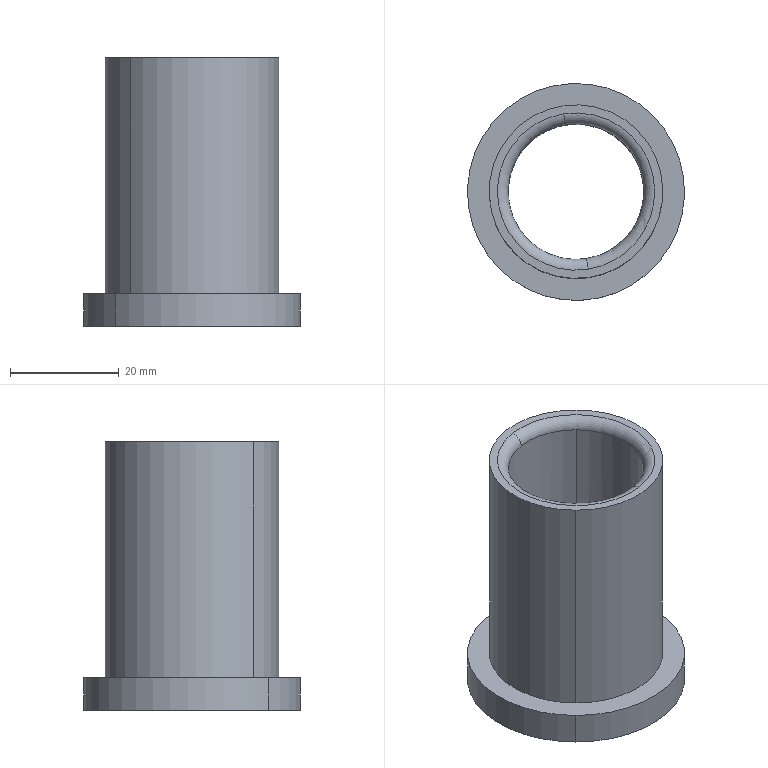Part | 1 solid | 11 faces | box 40 x 40 x 49.5 mm | volume 18157 mm3 | cylinder 6 | plane 3 | torus 2 | commonest cylinder face diameters 25 x2 32 x2 40 x2
STEP:
#1=CARTESIAN_POINT('',(0.,0.,0.));
#2=DIRECTION('',(0.,0.,1.));
#3=DIRECTION('',(1.,0.,0.));
#4=AXIS2_PLACEMENT_3D('',#1,#2,#3);
#5=CARTESIAN_POINT('',(-343.839,33.661,-238.55));
#6=VERTEX_POINT('',#5);
#7=CARTESIAN_POINT('',(-326.161,51.339,-238.55));
#8=VERTEX_POINT('',#7);
#9=CARTESIAN_POINT('',(-335.,42.5,-238.55));
#10=DIRECTION('',(0.,0.,1.));
#11=DIRECTION('',(0.7071,0.7071,0.));
#12=AXIS2_PLACEMENT_3D('',#9,#10,#11);
#13=CIRCLE('',#12,12.5);
#14=CARTESIAN_POINT('',(-335.,42.5,-200.318));
#15=DIRECTION('',(0.,0.,1.));
#16=DIRECTION('',(-0.7071,0.7071,0.));
#17=AXIS2_PLACEMENT_3D('',#14,#15,#16);
#18=CYLINDRICAL_SURFACE('',#17,12.5);
#19=CARTESIAN_POINT('',(-1.571,-38.232));
#20=DIRECTION('',(1.,0.));
#21=VECTOR('',#20,1.);
#22=LINE('',#19,#21);
#23=(GEOMETRIC_REPRESENTATION_CONTEXT(2)PARAMETRIC_REPRESENTATION_CONTEXT()REPRESENTATION_CONTEXT('',''));
#24=DEFINITIONAL_REPRESENTATION('',(#22),#23);
#25=PCURVE('',#18,#24);
#26=CARTESIAN_POINT('',(-320.858,28.358,-238.55));
#27=DIRECTION('',(0.,0.,-1.));
#28=DIRECTION('',(-0.7071,-0.7071,0.));
#29=AXIS2_PLACEMENT_3D('',#26,#27,#28);
#30=PLANE('',#29);
#31=CARTESIAN_POINT('',(-12.5,20.));
#32=CARTESIAN_POINT('',(-12.5,41.651));
#33=CARTESIAN_POINT('',(6.25,30.825));
#34=CARTESIAN_POINT('',(25.,20.));
#35=CARTESIAN_POINT('',(6.25,9.175));
#36=CARTESIAN_POINT('',(-12.5,-1.651));
#37=CARTESIAN_POINT('',(-12.5,20.));
#38=(BOUNDED_CURVE()B_SPLINE_CURVE(2,(#31,#32,#33,#34,#35,#36,#37),.UNSPECIFIED.,.T.,.F.)B_SPLINE_CURVE_WITH_KNOTS((1,2,2,2,2,1),(-2.094,0.,2.094,4.189,6.283,8.378),.UNSPECIFIED.)CURVE()GEOMETRIC_REPRESENTATION_ITEM()RATIONAL_B_SPLINE_CURVE((1.,0.5,1.,0.5,1.,0.5,1.))REPRESENTATION_ITEM(''));
#39=(GEOMETRIC_REPRESENTATION_CONTEXT(2)PARAMETRIC_REPRESENTATION_CONTEXT()REPRESENTATION_CONTEXT('',''));
#40=DEFINITIONAL_REPRESENTATION('',(#38),#39);
#41=PCURVE('',#30,#40);
#42=SURFACE_CURVE('',#13,(#25,#41),.PCURVE_S1.);
#43=EDGE_CURVE('',#6,#8,#42,.T.);
#44=ORIENTED_EDGE('',*,*,#43,.T.);
#45=CARTESIAN_POINT('',(-326.161,51.339,-191.05));
#46=VERTEX_POINT('',#45);
#47=CARTESIAN_POINT('',(-326.161,51.339,-238.55));
#48=DIRECTION('',(0.,0.,1.));
#49=VECTOR('',#48,1.);
#50=LINE('',#47,#49);
#51=CARTESIAN_POINT('',(4.712,-38.232));
#52=DIRECTION('',(0.,1.));
#53=VECTOR('',#52,1.);
#54=LINE('',#51,#53);
#55=(GEOMETRIC_REPRESENTATION_CONTEXT(2)PARAMETRIC_REPRESENTATION_CONTEXT()REPRESENTATION_CONTEXT('',''));
#56=DEFINITIONAL_REPRESENTATION('',(#54),#55);
#57=PCURVE('',#18,#56);
#58=CARTESIAN_POINT('',(-335.,42.5,-200.318));
#59=DIRECTION('',(0.,0.,1.));
#60=DIRECTION('',(0.7071,-0.7071,0.));
#61=AXIS2_PLACEMENT_3D('',#58,#59,#60);
#62=CYLINDRICAL_SURFACE('',#61,12.5);
#63=CARTESIAN_POINT('',(1.571,-38.232));
#64=DIRECTION('',(0.,1.));
#65=VECTOR('',#64,1.);
#66=LINE('',#63,#65);
#67=(GEOMETRIC_REPRESENTATION_CONTEXT(2)PARAMETRIC_REPRESENTATION_CONTEXT()REPRESENTATION_CONTEXT('',''));
#68=DEFINITIONAL_REPRESENTATION('',(#66),#67);
#69=PCURVE('',#62,#68);
#70=SURFACE_CURVE('',#50,(#57,#69),.PCURVE_S1.);
#71=EDGE_CURVE('',#8,#46,#70,.T.);
#72=ORIENTED_EDGE('',*,*,#71,.T.);
#73=CARTESIAN_POINT('',(-322.654,40.545,-191.05));
#74=VERTEX_POINT('',#73);
#75=CARTESIAN_POINT('',(-335.,42.5,-191.05));
#76=DIRECTION('',(0.,0.,-1.));
#77=DIRECTION('',(0.9877,-0.1564,0.));
#78=AXIS2_PLACEMENT_3D('',#75,#76,#77);
#79=CIRCLE('',#78,12.5);
#80=CARTESIAN_POINT('',(10.053,9.268));
#81=DIRECTION('',(-1.,0.));
#82=VECTOR('',#81,1.);
#83=LINE('',#80,#82);
#84=(GEOMETRIC_REPRESENTATION_CONTEXT(2)PARAMETRIC_REPRESENTATION_CONTEXT()REPRESENTATION_CONTEXT('',''));
#85=DEFINITIONAL_REPRESENTATION('',(#83),#84);
#86=PCURVE('',#18,#85);
#87=CARTESIAN_POINT('',(-335.,42.5,-191.05));
#88=DIRECTION('',(0.,0.,1.));
#89=DIRECTION('',(-0.9877,-0.1564,0.));
#90=AXIS2_PLACEMENT_3D('',#87,#88,#89);
#91=TOROIDAL_SURFACE('',#90,14.5,2.);
#92=CARTESIAN_POINT('',(9.111,3.142));
#93=DIRECTION('',(-1.,0.));
#94=VECTOR('',#93,1.);
#95=LINE('',#92,#94);
#96=(GEOMETRIC_REPRESENTATION_CONTEXT(2)PARAMETRIC_REPRESENTATION_CONTEXT()REPRESENTATION_CONTEXT('',''));
#97=DEFINITIONAL_REPRESENTATION('',(#95),#96);
#98=PCURVE('',#91,#97);
#99=SURFACE_CURVE('',#79,(#86,#98),.PCURVE_S1.);
#100=EDGE_CURVE('',#46,#74,#99,.T.);
#101=ORIENTED_EDGE('',*,*,#100,.T.);
#102=CARTESIAN_POINT('',(-333.044,30.154,-191.05));
#103=VERTEX_POINT('',#102);
#104=CARTESIAN_POINT('',(-335.,42.5,-191.05));
#105=DIRECTION('',(0.,0.,-1.));
#106=DIRECTION('',(0.9877,-0.1564,0.));
#107=AXIS2_PLACEMENT_3D('',#104,#105,#106);
#108=CIRCLE('',#107,12.5);
#109=CARTESIAN_POINT('',(3.77,9.268));
#110=DIRECTION('',(-1.,0.));
#111=VECTOR('',#110,1.);
#112=LINE('',#109,#111);
#113=(GEOMETRIC_REPRESENTATION_CONTEXT(2)PARAMETRIC_REPRESENTATION_CONTEXT()REPRESENTATION_CONTEXT('',''));
#114=DEFINITIONAL_REPRESENTATION('',(#112),#113);
#115=PCURVE('',#18,#114);
#116=CARTESIAN_POINT('',(2.827,3.142));
#117=DIRECTION('',(-1.,0.));
#118=VECTOR('',#117,1.);
#119=LINE('',#116,#118);
#120=(GEOMETRIC_REPRESENTATION_CONTEXT(2)PARAMETRIC_REPRESENTATION_CONTEXT()REPRESENTATION_CONTEXT('',''));
#121=DEFINITIONAL_REPRESENTATION('',(#119),#120);
#122=PCURVE('',#91,#121);
#123=SURFACE_CURVE('',#108,(#115,#122),.PCURVE_S1.);
#124=EDGE_CURVE('',#74,#103,#123,.T.);
#125=ORIENTED_EDGE('',*,*,#124,.T.);
#126=CARTESIAN_POINT('',(-343.839,33.661,-191.05));
#127=VERTEX_POINT('',#126);
#128=CARTESIAN_POINT('',(-335.,42.5,-191.05));
#129=DIRECTION('',(0.,0.,-1.));
#130=DIRECTION('',(0.9877,-0.1564,0.));
#131=AXIS2_PLACEMENT_3D('',#128,#129,#130);
#132=CIRCLE('',#131,12.5);
#133=CARTESIAN_POINT('',(3.77,9.268));
#134=DIRECTION('',(-1.,0.));
#135=VECTOR('',#134,1.);
#136=LINE('',#133,#135);
#137=(GEOMETRIC_REPRESENTATION_CONTEXT(2)PARAMETRIC_REPRESENTATION_CONTEXT()REPRESENTATION_CONTEXT('',''));
#138=DEFINITIONAL_REPRESENTATION('',(#136),#137);
#139=PCURVE('',#18,#138);
#140=CARTESIAN_POINT('',(-335.,42.5,-191.05));
#141=DIRECTION('',(0.,0.,1.));
#142=DIRECTION('',(0.9877,0.1564,0.));
#143=AXIS2_PLACEMENT_3D('',#140,#141,#142);
#144=TOROIDAL_SURFACE('',#143,14.5,2.);
#145=CARTESIAN_POINT('',(5.969,3.142));
#146=DIRECTION('',(-1.,0.));
#147=VECTOR('',#146,1.);
#148=LINE('',#145,#147);
#149=(GEOMETRIC_REPRESENTATION_CONTEXT(2)PARAMETRIC_REPRESENTATION_CONTEXT()REPRESENTATION_CONTEXT('',''));
#150=DEFINITIONAL_REPRESENTATION('',(#148),#149);
#151=PCURVE('',#144,#150);
#152=SURFACE_CURVE('',#132,(#139,#151),.PCURVE_S1.);
#153=EDGE_CURVE('',#103,#127,#152,.T.);
#154=ORIENTED_EDGE('',*,*,#153,.T.);
#155=CARTESIAN_POINT('',(-343.839,33.661,-238.55));
#156=DIRECTION('',(0.,0.,1.));
#157=VECTOR('',#156,1.);
#158=LINE('',#155,#157);
#159=CARTESIAN_POINT('',(1.571,-38.232));
#160=DIRECTION('',(0.,1.));
#161=VECTOR('',#160,1.);
#162=LINE('',#159,#161);
#163=(GEOMETRIC_REPRESENTATION_CONTEXT(2)PARAMETRIC_REPRESENTATION_CONTEXT()REPRESENTATION_CONTEXT('',''));
#164=DEFINITIONAL_REPRESENTATION('',(#162),#163);
#165=PCURVE('',#18,#164);
#166=CARTESIAN_POINT('',(4.712,-38.232));
#167=DIRECTION('',(0.,1.));
#168=VECTOR('',#167,1.);
#169=LINE('',#166,#168);
#170=(GEOMETRIC_REPRESENTATION_CONTEXT(2)PARAMETRIC_REPRESENTATION_CONTEXT()REPRESENTATION_CONTEXT('',''));
#171=DEFINITIONAL_REPRESENTATION('',(#169),#170);
#172=PCURVE('',#62,#171);
#173=SURFACE_CURVE('',#158,(#165,#172),.PCURVE_S1.);
#174=EDGE_CURVE('',#6,#127,#173,.T.);
#175=ORIENTED_EDGE('',*,*,#174,.F.);
#176=EDGE_LOOP('',(#44,#72,#101,#125,#154,#175));
#177=FACE_BOUND('',#176,.F.);
#178=ADVANCED_FACE('',(#177),#18,.F.);
#179=CARTESIAN_POINT('',(-332.731,28.179,-189.05));
#180=VERTEX_POINT('',#179);
#181=CARTESIAN_POINT('',(-332.731,28.179,-191.05));
#182=DIRECTION('',(0.9877,0.1564,0.));
#183=DIRECTION('',(-0.1564,0.9877,0.));
#184=AXIS2_PLACEMENT_3D('',#181,#182,#183);
#185=CIRCLE('',#184,2.);
#186=CARTESIAN_POINT('',(1.571,3.142));
#187=DIRECTION('',(0.,-1.));
#188=VECTOR('',#187,1.);
#189=LINE('',#186,#188);
#190=(GEOMETRIC_REPRESENTATION_CONTEXT(2)PARAMETRIC_REPRESENTATION_CONTEXT()REPRESENTATION_CONTEXT('',''));
#191=DEFINITIONAL_REPRESENTATION('',(#189),#190);
#192=PCURVE('',#91,#191);
#193=CARTESIAN_POINT('',(4.712,3.142));
#194=DIRECTION('',(0.,-1.));
#195=VECTOR('',#194,1.);
#196=LINE('',#193,#195);
#197=(GEOMETRIC_REPRESENTATION_CONTEXT(2)PARAMETRIC_REPRESENTATION_CONTEXT()REPRESENTATION_CONTEXT('',''));
#198=DEFINITIONAL_REPRESENTATION('',(#196),#197);
#199=PCURVE('',#144,#198);
#200=SURFACE_CURVE('',#185,(#192,#199),.PCURVE_S1.);
#201=EDGE_CURVE('',#103,#180,#200,.T.);
#202=ORIENTED_EDGE('',*,*,#201,.T.);
#203=CARTESIAN_POINT('',(-320.678,40.232,-189.05));
#204=VERTEX_POINT('',#203);
#205=CARTESIAN_POINT('',(-335.,42.5,-189.05));
#206=DIRECTION('',(0.,0.,1.));
#207=DIRECTION('',(0.9877,-0.1564,0.));
#208=AXIS2_PLACEMENT_3D('',#205,#206,#207);
#209=CIRCLE('',#208,14.5);
#210=CARTESIAN_POINT('',(-3.456,1.571));
#211=DIRECTION('',(1.,0.));
#212=VECTOR('',#211,1.);
#213=LINE('',#210,#212);
#214=(GEOMETRIC_REPRESENTATION_CONTEXT(2)PARAMETRIC_REPRESENTATION_CONTEXT()REPRESENTATION_CONTEXT('',''));
#215=DEFINITIONAL_REPRESENTATION('',(#213),#214);
#216=PCURVE('',#91,#215);
#217=CARTESIAN_POINT('',(-201.386,25.559,-189.05));
#218=DIRECTION('',(0.,0.,1.));
#219=DIRECTION('',(-0.7071,0.7071,0.));
#220=AXIS2_PLACEMENT_3D('',#217,#218,#219);
#221=PLANE('',#220);
#222=CARTESIAN_POINT('',(106.458,82.5));
#223=DIRECTION('',(-0.809,-0.5878));
#224=AXIS2_PLACEMENT_2D('',#222,#223);
#225=CIRCLE('',#224,14.5);
#226=(GEOMETRIC_REPRESENTATION_CONTEXT(2)PARAMETRIC_REPRESENTATION_CONTEXT()REPRESENTATION_CONTEXT('',''));
#227=DEFINITIONAL_REPRESENTATION('',(#225),#226);
#228=PCURVE('',#221,#227);
#229=SURFACE_CURVE('',#209,(#216,#228),.PCURVE_S1.);
#230=EDGE_CURVE('',#180,#204,#229,.T.);
#231=ORIENTED_EDGE('',*,*,#230,.T.);
#232=CARTESIAN_POINT('',(-337.268,56.821,-189.05));
#233=VERTEX_POINT('',#232);
#234=CARTESIAN_POINT('',(-335.,42.5,-189.05));
#235=DIRECTION('',(0.,0.,1.));
#236=DIRECTION('',(0.9877,-0.1564,0.));
#237=AXIS2_PLACEMENT_3D('',#234,#235,#236);
#238=CIRCLE('',#237,14.5);
#239=CARTESIAN_POINT('',(2.827,1.571));
#240=DIRECTION('',(1.,0.));
#241=VECTOR('',#240,1.);
#242=LINE('',#239,#241);
#243=(GEOMETRIC_REPRESENTATION_CONTEXT(2)PARAMETRIC_REPRESENTATION_CONTEXT()REPRESENTATION_CONTEXT('',''));
#244=DEFINITIONAL_REPRESENTATION('',(#242),#243);
#245=PCURVE('',#91,#244);
#246=CARTESIAN_POINT('',(106.458,82.5));
#247=DIRECTION('',(-0.809,-0.5878));
#248=AXIS2_PLACEMENT_2D('',#246,#247);
#249=CIRCLE('',#248,14.5);
#250=(GEOMETRIC_REPRESENTATION_CONTEXT(2)PARAMETRIC_REPRESENTATION_CONTEXT()REPRESENTATION_CONTEXT('',''));
#251=DEFINITIONAL_REPRESENTATION('',(#249),#250);
#252=PCURVE('',#221,#251);
#253=SURFACE_CURVE('',#238,(#245,#252),.PCURVE_S1.);
#254=EDGE_CURVE('',#204,#233,#253,.T.);
#255=ORIENTED_EDGE('',*,*,#254,.T.);
#256=CARTESIAN_POINT('',(-336.955,54.846,-191.05));
#257=VERTEX_POINT('',#256);
#258=CARTESIAN_POINT('',(-337.268,56.821,-191.05));
#259=DIRECTION('',(-0.9877,-0.1564,0.));
#260=DIRECTION('',(0.1564,-0.9877,0.));
#261=AXIS2_PLACEMENT_3D('',#258,#259,#260);
#262=CIRCLE('',#261,2.);
#263=CARTESIAN_POINT('',(4.712,3.142));
#264=DIRECTION('',(0.,-1.));
#265=VECTOR('',#264,1.);
#266=LINE('',#263,#265);
#267=(GEOMETRIC_REPRESENTATION_CONTEXT(2)PARAMETRIC_REPRESENTATION_CONTEXT()REPRESENTATION_CONTEXT('',''));
#268=DEFINITIONAL_REPRESENTATION('',(#266),#267);
#269=PCURVE('',#91,#268);
#270=CARTESIAN_POINT('',(1.571,3.142));
#271=DIRECTION('',(0.,-1.));
#272=VECTOR('',#271,1.);
#273=LINE('',#270,#272);
#274=(GEOMETRIC_REPRESENTATION_CONTEXT(2)PARAMETRIC_REPRESENTATION_CONTEXT()REPRESENTATION_CONTEXT('',''));
#275=DEFINITIONAL_REPRESENTATION('',(#273),#274);
#276=PCURVE('',#144,#275);
#277=SURFACE_CURVE('',#262,(#269,#276),.PCURVE_S1.);
#278=EDGE_CURVE('',#257,#233,#277,.T.);
#279=ORIENTED_EDGE('',*,*,#278,.F.);
#280=CARTESIAN_POINT('',(-335.,42.5,-191.05));
#281=DIRECTION('',(0.,0.,-1.));
#282=DIRECTION('',(0.9877,-0.1564,0.));
#283=AXIS2_PLACEMENT_3D('',#280,#281,#282);
#284=CIRCLE('',#283,12.5);
#285=CARTESIAN_POINT('',(9.111,3.142));
#286=DIRECTION('',(-1.,0.));
#287=VECTOR('',#286,1.);
#288=LINE('',#285,#287);
#289=(GEOMETRIC_REPRESENTATION_CONTEXT(2)PARAMETRIC_REPRESENTATION_CONTEXT()REPRESENTATION_CONTEXT('',''));
#290=DEFINITIONAL_REPRESENTATION('',(#288),#289);
#291=PCURVE('',#91,#290);
#292=CARTESIAN_POINT('',(6.912,9.268));
#293=DIRECTION('',(-1.,0.));
#294=VECTOR('',#293,1.);
#295=LINE('',#292,#294);
#296=(GEOMETRIC_REPRESENTATION_CONTEXT(2)PARAMETRIC_REPRESENTATION_CONTEXT()REPRESENTATION_CONTEXT('',''));
#297=DEFINITIONAL_REPRESENTATION('',(#295),#296);
#298=PCURVE('',#62,#297);
#299=SURFACE_CURVE('',#284,(#291,#298),.PCURVE_S1.);
#300=EDGE_CURVE('',#257,#46,#299,.T.);
#301=ORIENTED_EDGE('',*,*,#300,.T.);
#302=ORIENTED_EDGE('',*,*,#100,.T.);
#303=ORIENTED_EDGE('',*,*,#124,.T.);
#304=EDGE_LOOP('',(#202,#231,#255,#279,#301,#302,#303));
#305=FACE_BOUND('',#304,.T.);
#306=ADVANCED_FACE('',(#305),#91,.T.);
#307=ORIENTED_EDGE('',*,*,#230,.F.);
#308=CARTESIAN_POINT('',(-335.,42.5,-189.05));
#309=DIRECTION('',(0.,0.,1.));
#310=DIRECTION('',(0.9877,-0.1564,0.));
#311=AXIS2_PLACEMENT_3D('',#308,#309,#310);
#312=CIRCLE('',#311,14.5);
#313=CARTESIAN_POINT('',(106.458,82.5));
#314=DIRECTION('',(-0.809,-0.5878));
#315=AXIS2_PLACEMENT_2D('',#313,#314);
#316=CIRCLE('',#315,14.5);
#317=(GEOMETRIC_REPRESENTATION_CONTEXT(2)PARAMETRIC_REPRESENTATION_CONTEXT()REPRESENTATION_CONTEXT('',''));
#318=DEFINITIONAL_REPRESENTATION('',(#316),#317);
#319=PCURVE('',#221,#318);
#320=CARTESIAN_POINT('',(-0.3142,1.571));
#321=DIRECTION('',(1.,0.));
#322=VECTOR('',#321,1.);
#323=LINE('',#320,#322);
#324=(GEOMETRIC_REPRESENTATION_CONTEXT(2)PARAMETRIC_REPRESENTATION_CONTEXT()REPRESENTATION_CONTEXT('',''));
#325=DEFINITIONAL_REPRESENTATION('',(#323),#324);
#326=PCURVE('',#144,#325);
#327=SURFACE_CURVE('',#312,(#319,#326),.PCURVE_S1.);
#328=EDGE_CURVE('',#233,#180,#327,.T.);
#329=ORIENTED_EDGE('',*,*,#328,.F.);
#330=ORIENTED_EDGE('',*,*,#254,.F.);
#331=EDGE_LOOP('',(#307,#329,#330));
#332=FACE_BOUND('',#331,.T.);
#333=CARTESIAN_POINT('',(-323.686,53.814,-189.05));
#334=VERTEX_POINT('',#333);
#335=CARTESIAN_POINT('',(-346.313,31.186,-189.05));
#336=VERTEX_POINT('',#335);
#337=CARTESIAN_POINT('',(-335.,42.5,-189.05));
#338=DIRECTION('',(0.,0.,1.));
#339=DIRECTION('',(0.7071,0.7071,0.));
#340=AXIS2_PLACEMENT_3D('',#337,#338,#339);
#341=CIRCLE('',#340,16.);
#342=CARTESIAN_POINT('',(106.458,82.5));
#343=DIRECTION('',(0.,-1.));
#344=AXIS2_PLACEMENT_2D('',#342,#343);
#345=CIRCLE('',#344,16.);
#346=(GEOMETRIC_REPRESENTATION_CONTEXT(2)PARAMETRIC_REPRESENTATION_CONTEXT()REPRESENTATION_CONTEXT('',''));
#347=DEFINITIONAL_REPRESENTATION('',(#345),#346);
#348=PCURVE('',#221,#347);
#349=CARTESIAN_POINT('',(-335.,42.5,-200.318));
#350=DIRECTION('',(0.,0.,1.));
#351=DIRECTION('',(0.7071,-0.7071,0.));
#352=AXIS2_PLACEMENT_3D('',#349,#350,#351);
#353=CYLINDRICAL_SURFACE('',#352,16.);
#354=CARTESIAN_POINT('',(1.571,11.268));
#355=DIRECTION('',(1.,0.));
#356=VECTOR('',#355,1.);
#357=LINE('',#354,#356);
#358=(GEOMETRIC_REPRESENTATION_CONTEXT(2)PARAMETRIC_REPRESENTATION_CONTEXT()REPRESENTATION_CONTEXT('',''));
#359=DEFINITIONAL_REPRESENTATION('',(#357),#358);
#360=PCURVE('',#353,#359);
#361=SURFACE_CURVE('',#341,(#348,#360),.PCURVE_S1.);
#362=EDGE_CURVE('',#334,#336,#361,.T.);
#363=ORIENTED_EDGE('',*,*,#362,.T.);
#364=CARTESIAN_POINT('',(-335.,42.5,-189.05));
#365=DIRECTION('',(0.,0.,1.));
#366=DIRECTION('',(0.7071,0.7071,0.));
#367=AXIS2_PLACEMENT_3D('',#364,#365,#366);
#368=CIRCLE('',#367,16.);
#369=CARTESIAN_POINT('',(106.458,82.5));
#370=DIRECTION('',(0.,-1.));
#371=AXIS2_PLACEMENT_2D('',#369,#370);
#372=CIRCLE('',#371,16.);
#373=(GEOMETRIC_REPRESENTATION_CONTEXT(2)PARAMETRIC_REPRESENTATION_CONTEXT()REPRESENTATION_CONTEXT('',''));
#374=DEFINITIONAL_REPRESENTATION('',(#372),#373);
#375=PCURVE('',#221,#374);
#376=CARTESIAN_POINT('',(-335.,42.5,-200.318));
#377=DIRECTION('',(0.,0.,1.));
#378=DIRECTION('',(-0.7071,0.7071,0.));
#379=AXIS2_PLACEMENT_3D('',#376,#377,#378);
#380=CYLINDRICAL_SURFACE('',#379,16.);
#381=CARTESIAN_POINT('',(-1.571,11.268));
#382=DIRECTION('',(1.,0.));
#383=VECTOR('',#382,1.);
#384=LINE('',#381,#383);
#385=(GEOMETRIC_REPRESENTATION_CONTEXT(2)PARAMETRIC_REPRESENTATION_CONTEXT()REPRESENTATION_CONTEXT('',''));
#386=DEFINITIONAL_REPRESENTATION('',(#384),#385);
#387=PCURVE('',#380,#386);
#388=SURFACE_CURVE('',#368,(#375,#387),.PCURVE_S1.);
#389=EDGE_CURVE('',#336,#334,#388,.T.);
#390=ORIENTED_EDGE('',*,*,#389,.T.);
#391=EDGE_LOOP('',(#363,#390));
#392=FACE_BOUND('',#391,.T.);
#393=ADVANCED_FACE('',(#332,#392),#221,.T.);
#394=CARTESIAN_POINT('',(-346.313,31.186,-232.55));
#395=VERTEX_POINT('',#394);
#396=CARTESIAN_POINT('',(-346.313,31.186,-232.55));
#397=DIRECTION('',(0.,0.,1.));
#398=VECTOR('',#397,1.);
#399=LINE('',#396,#398);
#400=CARTESIAN_POINT('',(1.571,-32.232));
#401=DIRECTION('',(0.,1.));
#402=VECTOR('',#401,1.);
#403=LINE('',#400,#402);
#404=(GEOMETRIC_REPRESENTATION_CONTEXT(2)PARAMETRIC_REPRESENTATION_CONTEXT()REPRESENTATION_CONTEXT('',''));
#405=DEFINITIONAL_REPRESENTATION('',(#403),#404);
#406=PCURVE('',#380,#405);
#407=CARTESIAN_POINT('',(4.712,-32.232));
#408=DIRECTION('',(0.,1.));
#409=VECTOR('',#408,1.);
#410=LINE('',#407,#409);
#411=(GEOMETRIC_REPRESENTATION_CONTEXT(2)PARAMETRIC_REPRESENTATION_CONTEXT()REPRESENTATION_CONTEXT('',''));
#412=DEFINITIONAL_REPRESENTATION('',(#410),#411);
#413=PCURVE('',#353,#412);
#414=SURFACE_CURVE('',#399,(#406,#413),.PCURVE_S1.);
#415=EDGE_CURVE('',#395,#336,#414,.T.);
#416=ORIENTED_EDGE('',*,*,#415,.F.);
#417=CARTESIAN_POINT('',(-323.686,53.814,-232.55));
#418=VERTEX_POINT('',#417);
#419=CARTESIAN_POINT('',(-335.,42.5,-232.55));
#420=DIRECTION('',(0.,0.,1.));
#421=DIRECTION('',(0.7071,0.7071,0.));
#422=AXIS2_PLACEMENT_3D('',#419,#420,#421);
#423=CIRCLE('',#422,16.);
#424=CARTESIAN_POINT('',(-1.571,-32.232));
#425=DIRECTION('',(1.,0.));
#426=VECTOR('',#425,1.);
#427=LINE('',#424,#426);
#428=(GEOMETRIC_REPRESENTATION_CONTEXT(2)PARAMETRIC_REPRESENTATION_CONTEXT()REPRESENTATION_CONTEXT('',''));
#429=DEFINITIONAL_REPRESENTATION('',(#427),#428);
#430=PCURVE('',#380,#429);
#431=CARTESIAN_POINT('',(-323.686,31.186,-232.55));
#432=DIRECTION('',(0.,0.,1.));
#433=DIRECTION('',(0.7071,0.7071,0.));
#434=AXIS2_PLACEMENT_3D('',#431,#432,#433);
#435=PLANE('',#434);
#436=CARTESIAN_POINT('',(0.,16.));
#437=DIRECTION('',(1.,0.));
#438=AXIS2_PLACEMENT_2D('',#436,#437);
#439=CIRCLE('',#438,16.);
#440=(GEOMETRIC_REPRESENTATION_CONTEXT(2)PARAMETRIC_REPRESENTATION_CONTEXT()REPRESENTATION_CONTEXT('',''));
#441=DEFINITIONAL_REPRESENTATION('',(#439),#440);
#442=PCURVE('',#435,#441);
#443=SURFACE_CURVE('',#423,(#430,#442),.PCURVE_S1.);
#444=EDGE_CURVE('',#395,#418,#443,.T.);
#445=ORIENTED_EDGE('',*,*,#444,.T.);
#446=CARTESIAN_POINT('',(-323.686,53.814,-232.55));
#447=DIRECTION('',(0.,0.,1.));
#448=VECTOR('',#447,1.);
#449=LINE('',#446,#448);
#450=CARTESIAN_POINT('',(4.712,-32.232));
#451=DIRECTION('',(0.,1.));
#452=VECTOR('',#451,1.);
#453=LINE('',#450,#452);
#454=(GEOMETRIC_REPRESENTATION_CONTEXT(2)PARAMETRIC_REPRESENTATION_CONTEXT()REPRESENTATION_CONTEXT('',''));
#455=DEFINITIONAL_REPRESENTATION('',(#453),#454);
#456=PCURVE('',#380,#455);
#457=CARTESIAN_POINT('',(1.571,-32.232));
#458=DIRECTION('',(0.,1.));
#459=VECTOR('',#458,1.);
#460=LINE('',#457,#459);
#461=(GEOMETRIC_REPRESENTATION_CONTEXT(2)PARAMETRIC_REPRESENTATION_CONTEXT()REPRESENTATION_CONTEXT('',''));
#462=DEFINITIONAL_REPRESENTATION('',(#460),#461);
#463=PCURVE('',#353,#462);
#464=SURFACE_CURVE('',#449,(#456,#463),.PCURVE_S1.);
#465=EDGE_CURVE('',#418,#334,#464,.T.);
#466=ORIENTED_EDGE('',*,*,#465,.T.);
#467=ORIENTED_EDGE('',*,*,#389,.F.);
#468=EDGE_LOOP('',(#416,#445,#466,#467));
#469=FACE_BOUND('',#468,.T.);
#470=ADVANCED_FACE('',(#469),#380,.T.);
#471=CARTESIAN_POINT('',(-320.858,56.642,-232.55));
#472=VERTEX_POINT('',#471);
#473=CARTESIAN_POINT('',(-349.142,28.358,-232.55));
#474=VERTEX_POINT('',#473);
#475=CARTESIAN_POINT('',(-335.,42.5,-232.55));
#476=DIRECTION('',(0.,0.,1.));
#477=DIRECTION('',(0.7071,0.7071,0.));
#478=AXIS2_PLACEMENT_3D('',#475,#476,#477);
#479=CIRCLE('',#478,20.);
#480=CARTESIAN_POINT('',(0.,16.));
#481=DIRECTION('',(1.,0.));
#482=AXIS2_PLACEMENT_2D('',#480,#481);
#483=CIRCLE('',#482,20.);
#484=(GEOMETRIC_REPRESENTATION_CONTEXT(2)PARAMETRIC_REPRESENTATION_CONTEXT()REPRESENTATION_CONTEXT('',''));
#485=DEFINITIONAL_REPRESENTATION('',(#483),#484);
#486=PCURVE('',#435,#485);
#487=CARTESIAN_POINT('',(-335.,42.5,-200.318));
#488=DIRECTION('',(0.,0.,1.));
#489=DIRECTION('',(0.7071,-0.7071,0.));
#490=AXIS2_PLACEMENT_3D('',#487,#488,#489);
#491=CYLINDRICAL_SURFACE('',#490,20.);
#492=CARTESIAN_POINT('',(1.571,-32.232));
#493=DIRECTION('',(1.,0.));
#494=VECTOR('',#493,1.);
#495=LINE('',#492,#494);
#496=(GEOMETRIC_REPRESENTATION_CONTEXT(2)PARAMETRIC_REPRESENTATION_CONTEXT()REPRESENTATION_CONTEXT('',''));
#497=DEFINITIONAL_REPRESENTATION('',(#495),#496);
#498=PCURVE('',#491,#497);
#499=SURFACE_CURVE('',#479,(#486,#498),.PCURVE_S1.);
#500=EDGE_CURVE('',#472,#474,#499,.T.);
#501=ORIENTED_EDGE('',*,*,#500,.T.);
#502=CARTESIAN_POINT('',(-335.,42.5,-232.55));
#503=DIRECTION('',(0.,0.,1.));
#504=DIRECTION('',(0.7071,0.7071,0.));
#505=AXIS2_PLACEMENT_3D('',#502,#503,#504);
#506=CIRCLE('',#505,20.);
#507=CARTESIAN_POINT('',(0.,16.));
#508=DIRECTION('',(1.,0.));
#509=AXIS2_PLACEMENT_2D('',#507,#508);
#510=CIRCLE('',#509,20.);
#511=(GEOMETRIC_REPRESENTATION_CONTEXT(2)PARAMETRIC_REPRESENTATION_CONTEXT()REPRESENTATION_CONTEXT('',''));
#512=DEFINITIONAL_REPRESENTATION('',(#510),#511);
#513=PCURVE('',#435,#512);
#514=CARTESIAN_POINT('',(-335.,42.5,-200.318));
#515=DIRECTION('',(0.,0.,1.));
#516=DIRECTION('',(-0.7071,0.7071,0.));
#517=AXIS2_PLACEMENT_3D('',#514,#515,#516);
#518=CYLINDRICAL_SURFACE('',#517,20.);
#519=CARTESIAN_POINT('',(-1.571,-32.232));
#520=DIRECTION('',(1.,0.));
#521=VECTOR('',#520,1.);
#522=LINE('',#519,#521);
#523=(GEOMETRIC_REPRESENTATION_CONTEXT(2)PARAMETRIC_REPRESENTATION_CONTEXT()REPRESENTATION_CONTEXT('',''));
#524=DEFINITIONAL_REPRESENTATION('',(#522),#523);
#525=PCURVE('',#518,#524);
#526=SURFACE_CURVE('',#506,(#513,#525),.PCURVE_S1.);
#527=EDGE_CURVE('',#474,#472,#526,.T.);
#528=ORIENTED_EDGE('',*,*,#527,.T.);
#529=EDGE_LOOP('',(#501,#528));
#530=FACE_BOUND('',#529,.T.);
#531=ORIENTED_EDGE('',*,*,#444,.F.);
#532=CARTESIAN_POINT('',(-335.,42.5,-232.55));
#533=DIRECTION('',(0.,0.,1.));
#534=DIRECTION('',(0.7071,0.7071,0.));
#535=AXIS2_PLACEMENT_3D('',#532,#533,#534);
#536=CIRCLE('',#535,16.);
#537=CARTESIAN_POINT('',(0.,16.));
#538=DIRECTION('',(1.,0.));
#539=AXIS2_PLACEMENT_2D('',#537,#538);
#540=CIRCLE('',#539,16.);
#541=(GEOMETRIC_REPRESENTATION_CONTEXT(2)PARAMETRIC_REPRESENTATION_CONTEXT()REPRESENTATION_CONTEXT('',''));
#542=DEFINITIONAL_REPRESENTATION('',(#540),#541);
#543=PCURVE('',#435,#542);
#544=CARTESIAN_POINT('',(1.571,-32.232));
#545=DIRECTION('',(1.,0.));
#546=VECTOR('',#545,1.);
#547=LINE('',#544,#546);
#548=(GEOMETRIC_REPRESENTATION_CONTEXT(2)PARAMETRIC_REPRESENTATION_CONTEXT()REPRESENTATION_CONTEXT('',''));
#549=DEFINITIONAL_REPRESENTATION('',(#547),#548);
#550=PCURVE('',#353,#549);
#551=SURFACE_CURVE('',#536,(#543,#550),.PCURVE_S1.);
#552=EDGE_CURVE('',#418,#395,#551,.T.);
#553=ORIENTED_EDGE('',*,*,#552,.F.);
#554=EDGE_LOOP('',(#531,#553));
#555=FACE_BOUND('',#554,.T.);
#556=ADVANCED_FACE('',(#530,#555),#435,.T.);
#557=CARTESIAN_POINT('',(-349.142,28.358,-238.55));
#558=VERTEX_POINT('',#557);
#559=CARTESIAN_POINT('',(-349.142,28.358,-238.55));
#560=DIRECTION('',(0.,0.,1.));
#561=VECTOR('',#560,1.);
#562=LINE('',#559,#561);
#563=CARTESIAN_POINT('',(1.571,-38.232));
#564=DIRECTION('',(0.,1.));
#565=VECTOR('',#564,1.);
#566=LINE('',#563,#565);
#567=(GEOMETRIC_REPRESENTATION_CONTEXT(2)PARAMETRIC_REPRESENTATION_CONTEXT()REPRESENTATION_CONTEXT('',''));
#568=DEFINITIONAL_REPRESENTATION('',(#566),#567);
#569=PCURVE('',#518,#568);
#570=CARTESIAN_POINT('',(4.712,-38.232));
#571=DIRECTION('',(0.,1.));
#572=VECTOR('',#571,1.);
#573=LINE('',#570,#572);
#574=(GEOMETRIC_REPRESENTATION_CONTEXT(2)PARAMETRIC_REPRESENTATION_CONTEXT()REPRESENTATION_CONTEXT('',''));
#575=DEFINITIONAL_REPRESENTATION('',(#573),#574);
#576=PCURVE('',#491,#575);
#577=SURFACE_CURVE('',#562,(#569,#576),.PCURVE_S1.);
#578=EDGE_CURVE('',#558,#474,#577,.T.);
#579=ORIENTED_EDGE('',*,*,#578,.F.);
#580=CARTESIAN_POINT('',(-320.858,56.642,-238.55));
#581=VERTEX_POINT('',#580);
#582=CARTESIAN_POINT('',(-335.,42.5,-238.55));
#583=DIRECTION('',(0.,0.,1.));
#584=DIRECTION('',(0.7071,0.7071,0.));
#585=AXIS2_PLACEMENT_3D('',#582,#583,#584);
#586=CIRCLE('',#585,20.);
#587=CARTESIAN_POINT('',(-1.571,-38.232));
#588=DIRECTION('',(1.,0.));
#589=VECTOR('',#588,1.);
#590=LINE('',#587,#589);
#591=(GEOMETRIC_REPRESENTATION_CONTEXT(2)PARAMETRIC_REPRESENTATION_CONTEXT()REPRESENTATION_CONTEXT('',''));
#592=DEFINITIONAL_REPRESENTATION('',(#590),#591);
#593=PCURVE('',#518,#592);
#594=CARTESIAN_POINT('',(-20.,20.));
#595=CARTESIAN_POINT('',(-20.,54.641));
#596=CARTESIAN_POINT('',(10.,37.321));
#597=CARTESIAN_POINT('',(40.,20.));
#598=CARTESIAN_POINT('',(10.,2.679));
#599=CARTESIAN_POINT('',(-20.,-14.641));
#600=CARTESIAN_POINT('',(-20.,20.));
#601=(BOUNDED_CURVE()B_SPLINE_CURVE(2,(#594,#595,#596,#597,#598,#599,#600),.UNSPECIFIED.,.T.,.F.)B_SPLINE_CURVE_WITH_KNOTS((1,2,2,2,2,1),(-2.094,0.,2.094,4.189,6.283,8.378),.UNSPECIFIED.)CURVE()GEOMETRIC_REPRESENTATION_ITEM()RATIONAL_B_SPLINE_CURVE((1.,0.5,1.,0.5,1.,0.5,1.))REPRESENTATION_ITEM(''));
#602=(GEOMETRIC_REPRESENTATION_CONTEXT(2)PARAMETRIC_REPRESENTATION_CONTEXT()REPRESENTATION_CONTEXT('',''));
#603=DEFINITIONAL_REPRESENTATION('',(#601),#602);
#604=PCURVE('',#30,#603);
#605=SURFACE_CURVE('',#586,(#593,#604),.PCURVE_S1.);
#606=EDGE_CURVE('',#558,#581,#605,.T.);
#607=ORIENTED_EDGE('',*,*,#606,.T.);
#608=CARTESIAN_POINT('',(-320.858,56.642,-238.55));
#609=DIRECTION('',(0.,0.,1.));
#610=VECTOR('',#609,1.);
#611=LINE('',#608,#610);
#612=CARTESIAN_POINT('',(4.712,-38.232));
#613=DIRECTION('',(0.,1.));
#614=VECTOR('',#613,1.);
#615=LINE('',#612,#614);
#616=(GEOMETRIC_REPRESENTATION_CONTEXT(2)PARAMETRIC_REPRESENTATION_CONTEXT()REPRESENTATION_CONTEXT('',''));
#617=DEFINITIONAL_REPRESENTATION('',(#615),#616);
#618=PCURVE('',#518,#617);
#619=CARTESIAN_POINT('',(1.571,-38.232));
#620=DIRECTION('',(0.,1.));
#621=VECTOR('',#620,1.);
#622=LINE('',#619,#621);
#623=(GEOMETRIC_REPRESENTATION_CONTEXT(2)PARAMETRIC_REPRESENTATION_CONTEXT()REPRESENTATION_CONTEXT('',''));
#624=DEFINITIONAL_REPRESENTATION('',(#622),#623);
#625=PCURVE('',#491,#624);
#626=SURFACE_CURVE('',#611,(#618,#625),.PCURVE_S1.);
#627=EDGE_CURVE('',#581,#472,#626,.T.);
#628=ORIENTED_EDGE('',*,*,#627,.T.);
#629=ORIENTED_EDGE('',*,*,#527,.F.);
#630=EDGE_LOOP('',(#579,#607,#628,#629));
#631=FACE_BOUND('',#630,.T.);
#632=ADVANCED_FACE('',(#631),#518,.T.);
#633=ORIENTED_EDGE('',*,*,#606,.F.);
#634=CARTESIAN_POINT('',(-335.,42.5,-238.55));
#635=DIRECTION('',(0.,0.,1.));
#636=DIRECTION('',(0.7071,0.7071,0.));
#637=AXIS2_PLACEMENT_3D('',#634,#635,#636);
#638=CIRCLE('',#637,20.);
#639=CARTESIAN_POINT('',(-20.,20.));
#640=CARTESIAN_POINT('',(-20.,54.641));
#641=CARTESIAN_POINT('',(10.,37.321));
#642=CARTESIAN_POINT('',(40.,20.));
#643=CARTESIAN_POINT('',(10.,2.679));
#644=CARTESIAN_POINT('',(-20.,-14.641));
#645=CARTESIAN_POINT('',(-20.,20.));
#646=(BOUNDED_CURVE()B_SPLINE_CURVE(2,(#639,#640,#641,#642,#643,#644,#645),.UNSPECIFIED.,.T.,.F.)B_SPLINE_CURVE_WITH_KNOTS((1,2,2,2,2,1),(-2.094,0.,2.094,4.189,6.283,8.378),.UNSPECIFIED.)CURVE()GEOMETRIC_REPRESENTATION_ITEM()RATIONAL_B_SPLINE_CURVE((1.,0.5,1.,0.5,1.,0.5,1.))REPRESENTATION_ITEM(''));
#647=(GEOMETRIC_REPRESENTATION_CONTEXT(2)PARAMETRIC_REPRESENTATION_CONTEXT()REPRESENTATION_CONTEXT('',''));
#648=DEFINITIONAL_REPRESENTATION('',(#646),#647);
#649=PCURVE('',#30,#648);
#650=CARTESIAN_POINT('',(1.571,-38.232));
#651=DIRECTION('',(1.,0.));
#652=VECTOR('',#651,1.);
#653=LINE('',#650,#652);
#654=(GEOMETRIC_REPRESENTATION_CONTEXT(2)PARAMETRIC_REPRESENTATION_CONTEXT()REPRESENTATION_CONTEXT('',''));
#655=DEFINITIONAL_REPRESENTATION('',(#653),#654);
#656=PCURVE('',#491,#655);
#657=SURFACE_CURVE('',#638,(#649,#656),.PCURVE_S1.);
#658=EDGE_CURVE('',#581,#558,#657,.T.);
#659=ORIENTED_EDGE('',*,*,#658,.F.);
#660=EDGE_LOOP('',(#633,#659));
#661=FACE_BOUND('',#660,.T.);
#662=CARTESIAN_POINT('',(-335.,42.5,-238.55));
#663=DIRECTION('',(0.,0.,1.));
#664=DIRECTION('',(0.7071,0.7071,0.));
#665=AXIS2_PLACEMENT_3D('',#662,#663,#664);
#666=CIRCLE('',#665,12.5);
#667=CARTESIAN_POINT('',(-12.5,20.));
#668=CARTESIAN_POINT('',(-12.5,41.651));
#669=CARTESIAN_POINT('',(6.25,30.825));
#670=CARTESIAN_POINT('',(25.,20.));
#671=CARTESIAN_POINT('',(6.25,9.175));
#672=CARTESIAN_POINT('',(-12.5,-1.651));
#673=CARTESIAN_POINT('',(-12.5,20.));
#674=(BOUNDED_CURVE()B_SPLINE_CURVE(2,(#667,#668,#669,#670,#671,#672,#673),.UNSPECIFIED.,.T.,.F.)B_SPLINE_CURVE_WITH_KNOTS((1,2,2,2,2,1),(-2.094,0.,2.094,4.189,6.283,8.378),.UNSPECIFIED.)CURVE()GEOMETRIC_REPRESENTATION_ITEM()RATIONAL_B_SPLINE_CURVE((1.,0.5,1.,0.5,1.,0.5,1.))REPRESENTATION_ITEM(''));
#675=(GEOMETRIC_REPRESENTATION_CONTEXT(2)PARAMETRIC_REPRESENTATION_CONTEXT()REPRESENTATION_CONTEXT('',''));
#676=DEFINITIONAL_REPRESENTATION('',(#674),#675);
#677=PCURVE('',#30,#676);
#678=CARTESIAN_POINT('',(1.571,-38.232));
#679=DIRECTION('',(1.,0.));
#680=VECTOR('',#679,1.);
#681=LINE('',#678,#680);
#682=(GEOMETRIC_REPRESENTATION_CONTEXT(2)PARAMETRIC_REPRESENTATION_CONTEXT()REPRESENTATION_CONTEXT('',''));
#683=DEFINITIONAL_REPRESENTATION('',(#681),#682);
#684=PCURVE('',#62,#683);
#685=SURFACE_CURVE('',#666,(#677,#684),.PCURVE_S1.);
#686=EDGE_CURVE('',#8,#6,#685,.T.);
#687=ORIENTED_EDGE('',*,*,#686,.T.);
#688=ORIENTED_EDGE('',*,*,#43,.T.);
#689=EDGE_LOOP('',(#687,#688));
#690=FACE_BOUND('',#689,.T.);
#691=ADVANCED_FACE('',(#661,#690),#30,.T.);
#692=CARTESIAN_POINT('',(-335.,42.5,-191.05));
#693=DIRECTION('',(0.,0.,-1.));
#694=DIRECTION('',(0.9877,-0.1564,0.));
#695=AXIS2_PLACEMENT_3D('',#692,#693,#694);
#696=CIRCLE('',#695,12.5);
#697=CARTESIAN_POINT('',(6.912,9.268));
#698=DIRECTION('',(-1.,0.));
#699=VECTOR('',#698,1.);
#700=LINE('',#697,#699);
#701=(GEOMETRIC_REPRESENTATION_CONTEXT(2)PARAMETRIC_REPRESENTATION_CONTEXT()REPRESENTATION_CONTEXT('',''));
#702=DEFINITIONAL_REPRESENTATION('',(#700),#701);
#703=PCURVE('',#62,#702);
#704=CARTESIAN_POINT('',(5.969,3.142));
#705=DIRECTION('',(-1.,0.));
#706=VECTOR('',#705,1.);
#707=LINE('',#704,#706);
#708=(GEOMETRIC_REPRESENTATION_CONTEXT(2)PARAMETRIC_REPRESENTATION_CONTEXT()REPRESENTATION_CONTEXT('',''));
#709=DEFINITIONAL_REPRESENTATION('',(#707),#708);
#710=PCURVE('',#144,#709);
#711=SURFACE_CURVE('',#696,(#703,#710),.PCURVE_S1.);
#712=EDGE_CURVE('',#127,#257,#711,.T.);
#713=ORIENTED_EDGE('',*,*,#712,.T.);
#714=ORIENTED_EDGE('',*,*,#300,.T.);
#715=ORIENTED_EDGE('',*,*,#71,.F.);
#716=ORIENTED_EDGE('',*,*,#686,.T.);
#717=ORIENTED_EDGE('',*,*,#174,.T.);
#718=EDGE_LOOP('',(#713,#714,#715,#716,#717));
#719=FACE_BOUND('',#718,.F.);
#720=ADVANCED_FACE('',(#719),#62,.F.);
#721=ORIENTED_EDGE('',*,*,#201,.F.);
#722=ORIENTED_EDGE('',*,*,#153,.T.);
#723=ORIENTED_EDGE('',*,*,#712,.T.);
#724=ORIENTED_EDGE('',*,*,#278,.T.);
#725=ORIENTED_EDGE('',*,*,#328,.T.);
#726=EDGE_LOOP('',(#721,#722,#723,#724,#725));
#727=FACE_BOUND('',#726,.T.);
#728=ADVANCED_FACE('',(#727),#144,.T.);
#729=ORIENTED_EDGE('',*,*,#415,.T.);
#730=ORIENTED_EDGE('',*,*,#362,.F.);
#731=ORIENTED_EDGE('',*,*,#465,.F.);
#732=ORIENTED_EDGE('',*,*,#552,.T.);
#733=EDGE_LOOP('',(#729,#730,#731,#732));
#734=FACE_BOUND('',#733,.T.);
#735=ADVANCED_FACE('',(#734),#353,.T.);
#736=ORIENTED_EDGE('',*,*,#578,.T.);
#737=ORIENTED_EDGE('',*,*,#500,.F.);
#738=ORIENTED_EDGE('',*,*,#627,.F.);
#739=ORIENTED_EDGE('',*,*,#658,.T.);
#740=EDGE_LOOP('',(#736,#737,#738,#739));
#741=FACE_BOUND('',#740,.T.);
#742=ADVANCED_FACE('',(#741),#491,.T.);
#743=CLOSED_SHELL('',(#178,#306,#393,#470,#556,#632,#691,#720,#728,#735,#742));
#744=MANIFOLD_SOLID_BREP('',#743);
#745=(LENGTH_UNIT()NAMED_UNIT(*)SI_UNIT(.MILLI.,.METRE.));
#746=UNCERTAINTY_MEASURE_WITH_UNIT(LENGTH_MEASURE(0.0000001),#745,'','');
#747=(NAMED_UNIT(*)PLANE_ANGLE_UNIT()SI_UNIT($,.RADIAN.));
#748=(NAMED_UNIT(*)SI_UNIT($,.STERADIAN.)SOLID_ANGLE_UNIT());
#749=(GEOMETRIC_REPRESENTATION_CONTEXT(3)GLOBAL_UNCERTAINTY_ASSIGNED_CONTEXT((#746))GLOBAL_UNIT_ASSIGNED_CONTEXT((#745,#747,#748))REPRESENTATION_CONTEXT('',''));
#750=ADVANCED_BREP_SHAPE_REPRESENTATION('',(#4,#744),#749);